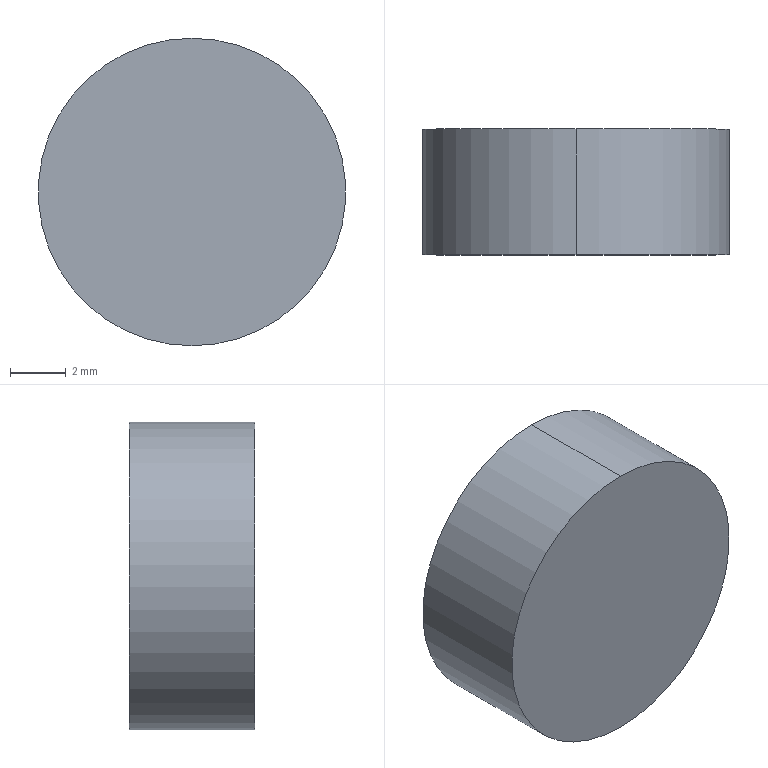Part | SolidWorks | features BaseBody 1 | 1 solid | 4 faces | box 11 x 4.5 x 11 mm | volume 427.649 mm3 | cylinder 2 | plane 2 | commonest cylinder face diameters 11 x2
STEP:
#1=CARTESIAN_POINT('',(0.,0.,5.5));
#2=VERTEX_POINT('',#1);
#3=CARTESIAN_POINT('',(0.,0.,-5.5));
#4=VERTEX_POINT('',#3);
#5=CARTESIAN_POINT('',(0.,0.,0.));
#6=DIRECTION('',(0.,1.,0.));
#7=DIRECTION('',(0.,0.,1.));
#8=AXIS2_PLACEMENT_3D('',#5,#6,#7);
#9=CIRCLE('',#8,5.5);
#10=EDGE_CURVE('',#2,#4,#9,.T.);
#11=ORIENTED_EDGE('',*,*,#10,.T.);
#12=CARTESIAN_POINT('',(0.,4.5,-5.5));
#13=VERTEX_POINT('',#12);
#14=CARTESIAN_POINT('',(0.,0.,-5.5));
#15=DIRECTION('',(0.,1.,0.));
#16=VECTOR('',#15,1000.);
#17=LINE('',#14,#16);
#18=EDGE_CURVE('',#4,#13,#17,.T.);
#19=ORIENTED_EDGE('',*,*,#18,.T.);
#20=CARTESIAN_POINT('',(0.,4.5,5.5));
#21=VERTEX_POINT('',#20);
#22=CARTESIAN_POINT('',(0.,4.5,0.));
#23=DIRECTION('',(0.,-1.,0.));
#24=DIRECTION('',(0.,0.,1.));
#25=AXIS2_PLACEMENT_3D('',#22,#23,#24);
#26=CIRCLE('',#25,5.5);
#27=EDGE_CURVE('',#13,#21,#26,.T.);
#28=ORIENTED_EDGE('',*,*,#27,.T.);
#29=CARTESIAN_POINT('',(0.,0.,5.5));
#30=DIRECTION('',(0.,1.,0.));
#31=VECTOR('',#30,1000.);
#32=LINE('',#29,#31);
#33=EDGE_CURVE('',#2,#21,#32,.T.);
#34=ORIENTED_EDGE('',*,*,#33,.F.);
#35=EDGE_LOOP('',(#11,#19,#28,#34));
#36=FACE_OUTER_BOUND('',#35,.T.);
#37=CARTESIAN_POINT('',(0.,0.,0.));
#38=DIRECTION('',(0.,1.,0.));
#39=DIRECTION('',(0.,0.,1.));
#40=AXIS2_PLACEMENT_3D('',#37,#38,#39);
#41=CYLINDRICAL_SURFACE('',#40,5.5);
#42=ADVANCED_FACE('',(#36),#41,.T.);
#43=ORIENTED_EDGE('',*,*,#18,.F.);
#44=CARTESIAN_POINT('',(0.,0.,0.));
#45=DIRECTION('',(0.,1.,0.));
#46=DIRECTION('',(0.,0.,1.));
#47=AXIS2_PLACEMENT_3D('',#44,#45,#46);
#48=CIRCLE('',#47,5.5);
#49=EDGE_CURVE('',#4,#2,#48,.T.);
#50=ORIENTED_EDGE('',*,*,#49,.T.);
#51=ORIENTED_EDGE('',*,*,#33,.T.);
#52=CARTESIAN_POINT('',(0.,4.5,0.));
#53=DIRECTION('',(0.,-1.,0.));
#54=DIRECTION('',(0.,0.,1.));
#55=AXIS2_PLACEMENT_3D('',#52,#53,#54);
#56=CIRCLE('',#55,5.5);
#57=EDGE_CURVE('',#21,#13,#56,.T.);
#58=ORIENTED_EDGE('',*,*,#57,.T.);
#59=EDGE_LOOP('',(#43,#50,#51,#58));
#60=FACE_OUTER_BOUND('',#59,.T.);
#61=CARTESIAN_POINT('',(0.,0.,0.));
#62=DIRECTION('',(0.,1.,0.));
#63=DIRECTION('',(0.,0.,1.));
#64=AXIS2_PLACEMENT_3D('',#61,#62,#63);
#65=CYLINDRICAL_SURFACE('',#64,5.5);
#66=ADVANCED_FACE('',(#60),#65,.T.);
#67=ORIENTED_EDGE('',*,*,#57,.F.);
#68=ORIENTED_EDGE('',*,*,#27,.F.);
#69=EDGE_LOOP('',(#67,#68));
#70=FACE_OUTER_BOUND('',#69,.T.);
#71=CARTESIAN_POINT('',(0.,4.5,0.));
#72=DIRECTION('',(0.,-1.,0.));
#73=DIRECTION('',(0.,0.,-1.));
#74=AXIS2_PLACEMENT_3D('',#71,#72,#73);
#75=PLANE('',#74);
#76=ADVANCED_FACE('',(#70),#75,.F.);
#77=ORIENTED_EDGE('',*,*,#10,.F.);
#78=ORIENTED_EDGE('',*,*,#49,.F.);
#79=EDGE_LOOP('',(#77,#78));
#80=FACE_OUTER_BOUND('',#79,.T.);
#81=CARTESIAN_POINT('',(5.5,0.,0.));
#82=DIRECTION('',(0.,1.,0.));
#83=DIRECTION('',(0.,0.,1.));
#84=AXIS2_PLACEMENT_3D('',#81,#82,#83);
#85=PLANE('',#84);
#86=ADVANCED_FACE('',(#80),#85,.F.);
#87=CLOSED_SHELL('',(#42,#66,#76,#86));
#88=MANIFOLD_SOLID_BREP('',#87);
#89=CARTESIAN_POINT('',(0.,0.,0.));
#90=DIRECTION('',(0.,0.,1.));
#91=DIRECTION('',(1.,0.,0.));
#92=AXIS2_PLACEMENT_3D('',#89,#90,#91);
#93=(LENGTH_UNIT()NAMED_UNIT(*)SI_UNIT(.MILLI.,.METRE.));
#94=UNCERTAINTY_MEASURE_WITH_UNIT(LENGTH_MEASURE(0.00001),#93,'','');
#95=(NAMED_UNIT(*)PLANE_ANGLE_UNIT()SI_UNIT($,.RADIAN.));
#96=(NAMED_UNIT(*)SI_UNIT($,.STERADIAN.)SOLID_ANGLE_UNIT());
#97=(GEOMETRIC_REPRESENTATION_CONTEXT(3)GLOBAL_UNCERTAINTY_ASSIGNED_CONTEXT((#94))GLOBAL_UNIT_ASSIGNED_CONTEXT((#93,#95,#96))REPRESENTATION_CONTEXT('',''));
#98=ADVANCED_BREP_SHAPE_REPRESENTATION('',(#88,#92),#97);